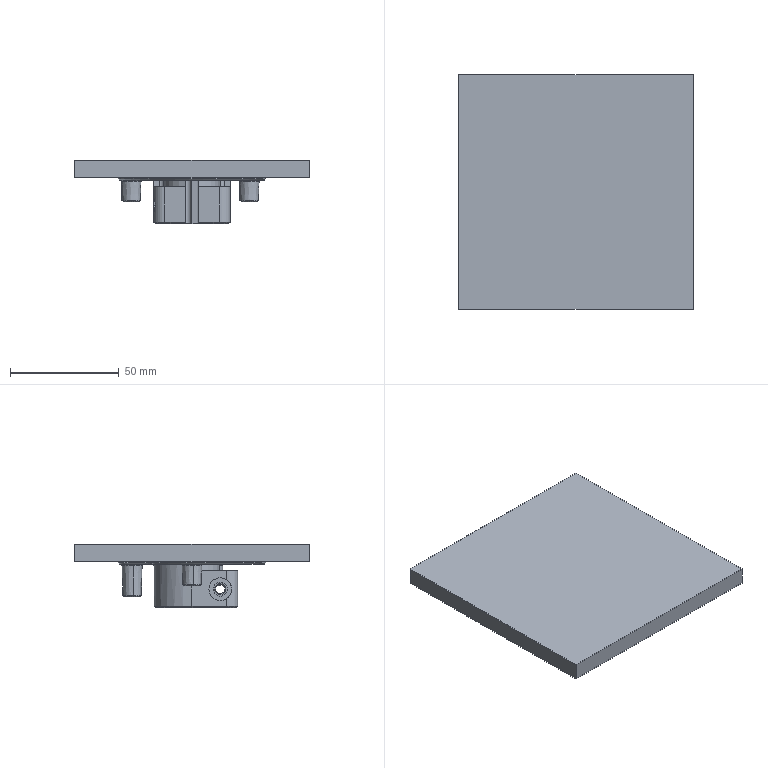NC program | NX | posted with a generic post | part box 108 x 108 x 29 mm
Lines 2749 to 3590 of 13118:
(ZLEVEL_PROFILE_COPY_COPY_COPY_1_COPY_COPY_1 , TOOL : D6JING)
N5466 T16 M6
N5468 G54
N5470 G17 G0 G90 X-1.747 Y-5.057 S9500 M3
N5472 G43 Z30. H16
N5474 Z-1.2
N5476 G94 G1 X-1.761 Y-5.965 F1000.
N5478 G3 X-1.468 Y-6.489 R0.6
N5480 G2 X0. Y-9.068 R3.013 F1500.
N5482 G1 X0.004 Y-9.036
N5484 X0.019 Y-8.767
N5486 X0.016 Y-8.756
N5488 G2 X1.421 Y-6.516 R3.
N5490 G3 X1.705 Y-5.987 R0.6
N5492 G1 X1.678 Y-5.08
N5494 G0 X-1.747 Y-5.057 Z-1.6
N5496 G1 X-1.761 Y-5.965 F1000.
N5498 G3 X-1.468 Y-6.489 R0.6
N5500 G2 X0. Y-9.068 R3.013 F1500.
N5502 G1 X0.004 Y-9.036
N5504 X0.019 Y-8.767
N5506 X0.016 Y-8.756
N5508 G2 X1.421 Y-6.515 R3.
N5510 G3 X1.706 Y-5.987 R0.6
N5512 G1 X1.678 Y-5.08
N5514 G0 X-1.747 Y-5.057 Z-2.
N5516 G1 X-1.76 Y-5.965 F1000.
N5518 G3 X-1.468 Y-6.489 R0.6
N5520 G2 X0. Y-9.068 R3.013 F1500.
N5522 G1 X0.004 Y-9.036
N5524 X0.019 Y-8.767
N5526 X0.016 Y-8.756
N5528 G2 X1.422 Y-6.515 R3.
N5530 G3 X1.706 Y-5.987 R0.6
N5532 G1 X1.678 Y-5.08
N5534 G0 X-1.747 Y-5.057 Z-2.4
N5536 G1 X-1.76 Y-5.965 F1000.
N5538 G3 X-1.468 Y-6.489 R0.6
N5540 G2 X0. Y-9.068 R3.013 F1500.
N5542 G1 X0.004 Y-9.036
N5544 X0.019 Y-8.767
N5546 X0.016 Y-8.756
N5548 G2 X1.422 Y-6.515 R3.
N5550 G3 X1.706 Y-5.987 R0.6
N5552 G1 X1.678 Y-5.08
N5554 G0 X-1.747 Y-5.057 Z-2.8
N5556 G1 X-1.76 Y-5.965 F1000.
N5558 G3 X-1.468 Y-6.489 R0.6
N5560 G2 X0. Y-9.068 R3.012 F1500.
N5562 G1 X0.004 Y-9.036
N5564 X0.018 Y-8.767
N5566 X0.016 Y-8.756
N5568 G2 X1.422 Y-6.515 R3.
N5570 G3 X1.706 Y-5.987 R0.6
N5572 G1 X1.679 Y-5.08
N5574 G0 X-1.747 Y-5.057 Z-3.2
N5576 G1 X-1.76 Y-5.965 F1000.
N5578 G3 X-1.468 Y-6.489 R0.6
N5580 G2 X0. Y-9.068 R3.012 F1500.
N5582 G1 X0.004 Y-9.036
N5584 X0.018 Y-8.767
N5586 X0.016 Y-8.756
N5588 G2 X1.422 Y-6.515 R3.
N5590 G3 X1.706 Y-5.987 R0.6
N5592 G1 X1.679 Y-5.08
N5594 G0 X-1.73 Y-5.062 Z-3.6
N5596 G1 X-1.746 Y-5.97 F1000.
N5598 G3 X-1.455 Y-6.495 R0.6
N5600 G2 X-0.016 Y-8.853 R2.983 F1500.
N5602 G1 X-0.001 Y-9.056
N5604 X0.003 Y-8.93
N5606 G2 X1.422 Y-6.515 R3.
N5608 G3 X1.706 Y-5.987 R0.6
N5610 G1 X1.679 Y-5.08
N5612 G0 X-1.73 Y-5.062 Z-4.
N5614 G1 X-1.746 Y-5.97 F1000.
N5616 G3 X-1.455 Y-6.495 R0.6
N5618 G2 X-0.016 Y-8.853 R2.983 F1500.
N5620 G1 X-0.001 Y-9.056
N5622 X0.003 Y-8.929
N5624 G2 X1.422 Y-6.515 R3.
N5626 G3 X1.707 Y-5.986 R0.6
N5628 G1 X1.679 Y-5.08
N5630 G0 X-1.73 Y-5.062 Z-4.4
N5632 G1 X-1.746 Y-5.97 F1000.
N5634 G3 X-1.455 Y-6.495 R0.6
N5636 G2 X-0.016 Y-8.853 R2.983 F1500.
N5638 G1 X-0.001 Y-9.056
N5640 X0.003 Y-8.928
N5642 G2 X1.422 Y-6.515 R3.
N5644 G3 X1.707 Y-5.986 R0.6
N5646 G1 X1.679 Y-5.08
N5648 G0 X-1.73 Y-5.062 Z-4.8
N5650 G1 X-1.746 Y-5.97 F1000.
N5652 G3 X-1.455 Y-6.495 R0.6
N5654 G2 X-0.016 Y-8.853 R2.983 F1500.
N5656 G1 X-0.001 Y-9.056
N5658 X0.003 Y-8.927
N5660 G2 X1.423 Y-6.515 R3.
N5662 G3 X1.707 Y-5.986 R0.6
N5664 G1 X1.68 Y-5.079
N5666 G0 X-1.73 Y-5.062 Z-5.2
N5668 G1 X-1.746 Y-5.97 F1000.
N5670 G3 X-1.455 Y-6.494 R0.6
N5672 G2 X-0.015 Y-8.853 R2.983 F1500.
N5674 G1 X-0.001 Y-9.056
N5676 X0.003 Y-8.925
N5678 G2 X1.423 Y-6.515 R3.
N5680 G3 X1.707 Y-5.986 R0.6
N5682 G1 X1.68 Y-5.079
N5684 G0 X-1.73 Y-5.062 Z-5.6
N5686 G1 X-1.746 Y-5.97 F1000.
N5688 G3 X-1.455 Y-6.494 R0.6
N5690 G2 X-0.015 Y-8.853 R2.983 F1500.
N5692 G1 X-0.001 Y-9.054
N5694 X0.004 Y-8.914
N5696 G2 X1.423 Y-6.515 R3.
N5698 G3 X1.707 Y-5.986 R0.6
N5700 G1 X1.68 Y-5.079
N5702 G0 X-1.73 Y-5.062 Z-6.
N5704 G1 X-1.746 Y-5.97 F1000.
N5706 G3 X-1.455 Y-6.494 R0.6
N5708 G2 X-0.015 Y-8.853 R2.983 F1500.
N5710 G1 X-0.001 Y-9.054
N5712 X0.004 Y-8.913
N5714 G2 X1.423 Y-6.514 R3.
N5716 G3 X1.707 Y-5.986 R0.6
N5718 G1 X1.68 Y-5.079
N5720 G0 X-1.731 Y-5.062 Z-6.4
N5722 G1 X-1.746 Y-5.97 F1000.
N5724 G3 X-1.455 Y-6.494 R0.6
N5726 G2 X-0.015 Y-8.853 R2.983 F1500.
N5728 G1 X-0.001 Y-9.054
N5730 X0.004 Y-8.912
N5732 G2 X1.423 Y-6.514 R3.
N5734 G3 X1.708 Y-5.986 R0.6
N5736 G1 X1.681 Y-5.079
N5738 G0 X-1.731 Y-5.062 Z-6.8
N5740 G1 X-1.746 Y-5.97 F1000.
N5742 G3 X-1.455 Y-6.494 R0.6
N5744 G2 X-0.015 Y-8.853 R2.983 F1500.
N5746 G1 X-0.001 Y-9.054
N5748 X0.004 Y-8.91
N5750 G2 X1.423 Y-6.514 R3.
N5752 G3 X1.708 Y-5.986 R0.6
N5754 G1 X1.681 Y-5.079
N5756 G0 X-1.731 Y-5.062 Z-7.2
N5758 G1 X-1.746 Y-5.97 F1000.
N5760 G3 X-1.455 Y-6.494 R0.6
N5762 G2 X-0.015 Y-8.853 R2.983 F1500.
N5764 G1 X-0.001 Y-9.053
N5766 X0.004 Y-8.908
N5768 G2 X1.424 Y-6.514 R3.
N5770 G3 X1.708 Y-5.986 R0.6
N5772 G1 X1.681 Y-5.079
N5774 G0 X-1.728 Y-5.063 Z-7.6
N5776 G1 X-1.744 Y-5.971 F1000.
N5778 G3 X-1.453 Y-6.495 R0.6
N5780 G2 X-0.013 Y-8.832 R2.988 F1500.
N5782 X-0.001 Y-9.06 R5.117
N5784 G1 X0.004 Y-8.915
N5786 G2 X1.424 Y-6.514 R3.
N5788 G3 X1.708 Y-5.986 R0.6
N5790 G1 X1.681 Y-5.079
N5792 G0 X-1.728 Y-5.063 Z-8.
N5794 G1 X-1.744 Y-5.971 F1000.
N5796 G3 X-1.453 Y-6.495 R0.6
N5798 G2 X-0.013 Y-8.833 R2.988 F1500.
N5800 X-0.001 Y-9.059 R5.079
N5802 G1 X0.004 Y-8.912
N5804 G2 X1.424 Y-6.514 R3.
N5806 G3 X1.708 Y-5.986 R0.6
N5808 G1 X1.681 Y-5.079
N5810 G0 X-1.728 Y-5.063 Z-8.4
N5812 G1 X-1.744 Y-5.971 F1000.
N5814 G3 X-1.454 Y-6.495 R0.6
N5816 G2 X-0.013 Y-8.833 R2.989 F1500.
N5818 X-0.001 Y-9.059 R5.041
N5820 G1 X0.004 Y-8.909
N5822 G2 X1.424 Y-6.514 R3.
N5824 G3 X1.708 Y-5.986 R0.6
N5826 G1 X1.682 Y-5.079
N5828 G0 X-1.728 Y-5.063 Z-8.8
N5830 G1 X-1.744 Y-5.97 F1000.
N5832 G3 X-1.454 Y-6.495 R0.6
N5834 G2 X-0.013 Y-8.833 R2.989 F1500.
N5836 X-0.001 Y-9.058 R5.003
N5838 G1 X0.004 Y-8.907
N5840 G2 X1.424 Y-6.514 R3.
N5842 G3 X1.709 Y-5.986 R0.6
N5844 G1 X1.682 Y-5.079
N5846 G0 X-1.729 Y-5.063 Z-9.2
N5848 G1 X-1.745 Y-5.97 F1000.
N5850 G3 X-1.454 Y-6.495 R0.6
N5852 G2 X-0.013 Y-8.834 R2.989 F1500.
N5854 X-0.001 Y-9.058 R4.964
N5856 G1 X0.004 Y-8.904
N5858 G2 X1.424 Y-6.514 R3.
N5860 G3 X1.709 Y-5.986 R0.6
N5862 G1 X1.682 Y-5.079
N5864 G0 X-1.729 Y-5.063 Z-9.6
N5866 G1 X-1.745 Y-5.97 F1000.
N5868 G3 X-1.454 Y-6.495 R0.6
N5870 G2 X-0.013 Y-8.834 R2.989 F1500.
N5872 X-0.001 Y-9.057 R4.926
N5874 G1 X0.005 Y-8.901
N5876 G2 X1.424 Y-6.514 R3.
N5878 G3 X1.709 Y-5.985 R0.6
N5880 G1 X1.682 Y-5.079
N5882 G0 X-1.729 Y-5.063 Z-10.
N5884 G1 X-1.745 Y-5.97 F1000.
N5886 G3 X-1.454 Y-6.495 R0.6
N5888 G2 X-0.013 Y-8.834 R2.989 F1500.
N5890 X-0.001 Y-9.057 R4.887
N5892 G1 X0.005 Y-8.899
N5894 G2 X1.425 Y-6.514 R3.
N5896 G3 X1.709 Y-5.985 R0.6
N5898 G1 X1.683 Y-5.079
N5900 G0 X-1.736 Y-5.061 Z-10.4
N5902 G1 X-1.751 Y-5.968 F1000.
N5904 G3 X-1.459 Y-6.493 R0.6
N5906 G2 X-0.012 Y-8.843 R2.994 F1500.
N5908 X-0.001 Y-9.057 R4.848
N5910 G1 X0.005 Y-8.896
N5912 G2 X1.425 Y-6.513 R3.
N5914 G3 X1.709 Y-5.985 R0.6
N5916 G1 X1.683 Y-5.078
N5918 G0 X-1.736 Y-5.061 Z-10.8
N5920 G1 X-1.751 Y-5.968 F1000.
N5922 G3 X-1.459 Y-6.493 R0.6
N5924 G2 X-0.012 Y-8.843 R2.994 F1500.
N5926 X-0.001 Y-9.056 R4.808
N5928 G1 X0.005 Y-8.893
N5930 G2 X1.425 Y-6.513 R3.
N5932 G3 X1.71 Y-5.985 R0.6
N5934 G1 X1.683 Y-5.078
N5936 G0 X-1.736 Y-5.061 Z-11.2
N5938 G1 X-1.751 Y-5.968 F1000.
N5940 G3 X-1.459 Y-6.493 R0.6
N5942 G2 X-0.012 Y-8.844 R2.994 F1500.
N5944 X-0.001 Y-9.056 R4.769
N5946 G1 X0.005 Y-8.891
N5948 G2 X1.425 Y-6.513 R3.
N5950 G3 X1.71 Y-5.985 R0.6
N5952 G1 X1.683 Y-5.078
N5954 G0 X-1.736 Y-5.06 Z-11.6
N5956 G1 X-1.751 Y-5.968 F1000.
N5958 G3 X-1.459 Y-6.493 R0.6
N5960 G2 X-0.012 Y-8.844 R2.994 F1500.
N5962 X-0.001 Y-9.056 R4.729
N5964 G1 X0.005 Y-8.89
N5966 G2 X1.425 Y-6.513 R3.
N5968 G3 X1.71 Y-5.985 R0.6
N5970 G1 X1.683 Y-5.078
N5972 G0 X-1.736 Y-5.06 Z-12.
N5974 G1 X-1.751 Y-5.968 F1000.
N5976 G3 X-1.459 Y-6.493 R0.6
N5978 G2 X-0.012 Y-8.845 R2.994 F1500.
N5980 X-0.001 Y-9.054 R4.69
N5982 G1 X0.006 Y-8.879
N5984 G2 X1.425 Y-6.513 R3.
N5986 G3 X1.71 Y-5.985 R0.6
N5988 G1 X1.684 Y-5.078
N5990 G0 X-1.736 Y-5.06 Z-12.4
N5992 G1 X-1.751 Y-5.968 F1000.
N5994 G3 X-1.459 Y-6.492 R0.6
N5996 G2 X-0.012 Y-8.845 R2.994 F1500.
N5998 X-0.001 Y-9.055 R4.649
N6000 G1 X0.006 Y-8.879
N6002 G2 X1.425 Y-6.513 R3.
N6004 G3 X1.71 Y-5.985 R0.6
N6006 G1 X1.684 Y-5.078
N6008 G0 X-1.736 Y-5.06 Z-12.8
N6010 G1 X-1.751 Y-5.968 F1000.
N6012 G3 X-1.459 Y-6.492 R0.6
N6014 G2 X-0.012 Y-8.845 R2.994 F1500.
N6016 X-0.001 Y-9.055 R4.609
N6018 G1 X0.006 Y-8.879
N6020 G2 X1.426 Y-6.513 R3.
N6022 G3 X1.71 Y-5.985 R0.6
N6024 G1 X1.684 Y-5.078
N6026 G0 X-1.778 Y-5.046 Z-13.2
N6028 G1 X-1.786 Y-5.956 F1000.
N6030 G3 X-1.491 Y-6.478 R0.6
N6032 G2 X0.001 Y-8.973 R3.033 F1500.
N6034 G1 X0.006 Y-8.881
N6036 G2 X1.426 Y-6.513 R3.
N6038 G3 X1.711 Y-5.985 R0.6
N6040 G1 X1.684 Y-5.078
N6042 G0 X-1.766 Y-5.05 Z-13.6
N6044 G1 X-1.776 Y-5.96 F1000.
N6046 G3 X-1.481 Y-6.482 R0.6
N6048 G2 X0.001 Y-8.971 R3.025 F1500.
N6050 G1 X0.006 Y-8.881
N6052 G2 X1.426 Y-6.513 R3.
N6054 G3 X1.711 Y-5.985 R0.6
N6056 G1 X1.685 Y-5.078
N6058 G0 X-1.745 Y-5.057 Z-14.
N6060 G1 X-1.758 Y-5.966 F1000.
N6062 G3 X-1.466 Y-6.49 R0.6
N6064 G2 X0. Y-9.067 R3.006 F1500.
N6066 G1 X0.017 Y-8.767
N6068 X0.016 Y-8.756
N6070 G2 X1.426 Y-6.513 R3.
N6072 G3 X1.711 Y-5.985 R0.6
N6074 G1 X1.685 Y-5.078
N6076 G0 X-1.745 Y-5.057 Z-14.4
N6078 G1 X-1.758 Y-5.966 F1000.
N6080 G3 X-1.465 Y-6.49 R0.6
N6082 G2 X0. Y-9.067 R3.006 F1500.
N6084 G1 X0.017 Y-8.767
N6086 X0.016 Y-8.756
N6088 G2 X1.426 Y-6.513 R3.
N6090 G3 X1.711 Y-5.985 R0.6
N6092 G1 X1.685 Y-5.078
N6094 G0 X-1.745 Y-5.058 Z-14.8
N6096 G1 X-1.758 Y-5.966 F1000.
N6098 G3 X-1.465 Y-6.49 R0.6
N6100 G2 X0. Y-9.067 R3.006 F1500.
N6102 G1 X0.017 Y-8.767
N6104 X0.016 Y-8.756
N6106 G2 X1.426 Y-6.512 R3.
N6108 G3 X1.711 Y-5.984 R0.6
N6110 G1 X1.685 Y-5.078
N6112 G0 X-1.745 Y-5.058 Z-15.2
N6114 G1 X-1.758 Y-5.966 F1000.
N6116 G3 X-1.465 Y-6.49 R0.6
N6118 G2 X0. Y-9.067 R3.006 F1500.
N6120 G1 X0.016 Y-8.756
N6122 G2 X1.426 Y-6.512 R3.
N6124 G3 X1.711 Y-5.984 R0.6
N6126 G1 X1.686 Y-5.078
N6128 G0 X-1.745 Y-5.058 Z-15.6
N6130 G1 X-1.758 Y-5.966 F1000.
N6132 G3 X-1.465 Y-6.49 R0.6
N6134 G2 X0. Y-9.067 R3.005 F1500.
N6136 G1 X0.016 Y-8.756
N6138 G2 X1.427 Y-6.512 R3.
N6140 G3 X1.712 Y-5.984 R0.6
N6142 G1 X1.686 Y-5.077
N6144 G0 X-1.745 Y-5.058 Z-16.
N6146 G1 X-1.758 Y-5.966 F1000.
N6148 G3 X-1.465 Y-6.49 R0.6
N6150 G2 X0. Y-9.066 R3.005 F1500.
N6152 G1 X0.016 Y-8.756
N6154 G2 X1.427 Y-6.512 R3.
N6156 G3 X1.712 Y-5.984 R0.6
N6158 G1 X1.686 Y-5.077
N6160 G0 X-1.744 Y-5.058 Z-16.4
N6162 G1 X-1.758 Y-5.966 F1000.
N6164 G3 X-1.465 Y-6.49 R0.6
N6166 G2 X0. Y-9.066 R3.005 F1500.
N6168 G1 X0.016 Y-8.756
N6170 G2 X1.427 Y-6.512 R3.
N6172 G3 X1.712 Y-5.984 R0.6
N6174 G1 X1.686 Y-5.077
N6176 G0 X-1.744 Y-5.058 Z-16.8
N6178 G1 X-1.757 Y-5.966 F1000.
N6180 G3 X-1.465 Y-6.49 R0.6
N6182 G2 X0. Y-9.066 R3.005 F1500.
N6184 G1 X0.016 Y-8.756
N6186 G2 X1.427 Y-6.512 R3.
N6188 G3 X1.712 Y-5.984 R0.6
N6190 G1 X1.686 Y-5.077
N6192 G0 X-1.744 Y-5.058 Z-17.2
N6194 G1 X-1.757 Y-5.966 F1000.
N6196 G3 X-1.465 Y-6.49 R0.6
N6198 G2 X0. Y-9.066 R3.004 F1500.
N6200 G1 X0.016 Y-8.756
N6202 G2 X1.427 Y-6.512 R3.
N6204 G3 X1.712 Y-5.984 R0.6
N6206 G1 X1.687 Y-5.077
N6208 G0 X-1.744 Y-5.058 Z-17.6
N6210 G1 X-1.757 Y-5.966 F1000.
N6212 G3 X-1.465 Y-6.49 R0.6
N6214 G2 X0. Y-9.066 R3.004 F1500.
N6216 G1 X0.016 Y-8.756
N6218 G2 X1.427 Y-6.512 R3.
N6220 G3 X1.713 Y-5.984 R0.6
N6222 G1 X1.687 Y-5.077
N6224 G0 X-1.744 Y-5.058 Z-18.
N6226 G1 X-1.757 Y-5.966 F1000.
N6228 G3 X-1.465 Y-6.49 R0.6
N6230 G2 X0. Y-9.066 R3.004 F1500.
N6232 G1 X0.016 Y-8.756
N6234 G2 X1.427 Y-6.512 R3.
N6236 G3 X1.713 Y-5.984 R0.6
N6238 G1 X1.687 Y-5.077
N6240 G0 X-1.744 Y-5.058 Z-18.4
N6242 G1 X-1.757 Y-5.966 F1000.
N6244 G3 X-1.465 Y-6.49 R0.6
N6246 G2 X0. Y-9.066 R3.004 F1500.
N6248 G1 X0.016 Y-8.756
N6250 G2 X1.428 Y-6.512 R3.
N6252 G3 X1.713 Y-5.984 R0.6
N6254 G1 X1.687 Y-5.077
N6256 G0 X-1.744 Y-5.058 Z-18.8
N6258 G1 X-1.757 Y-5.966 F1000.
N6260 G3 X-1.465 Y-6.49 R0.6
N6262 G2 X0. Y-9.066 R3.004 F1500.
N6264 G1 X0.016 Y-8.756
N6266 G2 X1.428 Y-6.512 R3.
N6268 G3 X1.713 Y-5.984 R0.6
N6270 G1 X1.688 Y-5.077
N6272 G0 X-1.744 Y-5.058 Z-19.2
N6274 G1 X-1.757 Y-5.966 F1000.
N6276 G3 X-1.464 Y-6.49 R0.6
N6278 G2 X0. Y-9.066 R3.003 F1500.
N6280 G1 X0.016 Y-8.756
N6282 G2 X1.428 Y-6.511 R3.
N6284 G3 X1.713 Y-5.984 R0.6
N6286 G1 X1.688 Y-5.077
N6288 G0 X-1.744 Y-5.058 Z-19.6
N6290 G1 X-1.757 Y-5.966 F1000.
N6292 G3 X-1.464 Y-6.49 R0.6
N6294 G2 X0. Y-9.066 R3.003 F1500.
N6296 G1 X0.016 Y-8.756
N6298 G2 X1.428 Y-6.511 R3.
N6300 G3 X1.713 Y-5.984 R0.6
N6302 G1 X1.688 Y-5.077
N6304 G0 X-1.744 Y-5.058 Z-20.
N6306 G1 X-1.757 Y-5.966 F1000.
N6308 G3 X-1.464 Y-6.49 R0.6
N6310 G2 X0. Y-9.066 R3.003 F1500.
N6312 G1 X0.016 Y-8.756
N6314 G2 X1.428 Y-6.511 R3.
N6316 G3 X1.714 Y-5.984 R0.6
N6318 G1 X1.688 Y-5.077
N6320 G0 X-1.744 Y-5.058 Z-20.4
N6322 G1 X-1.757 Y-5.966 F1000.
N6324 G3 X-1.464 Y-6.49 R0.6
N6326 G2 X0. Y-9.066 R3.003 F1500.
N6328 G1 X0.001 Y-9.036
N6330 X0.016 Y-8.756
N6332 G2 X1.428 Y-6.511 R3.
N6334 G3 X1.714 Y-5.983 R0.6
N6336 G1 X1.689 Y-5.077
N6338 G0 X-1.744 Y-5.058 Z-20.8
N6340 G1 X-1.757 Y-5.966 F1000.
N6342 G3 X-1.464 Y-6.49 R0.6
N6344 G2 X0. Y-9.066 R3.002 F1500.
N6346 G1 X0.001 Y-9.036
N6348 X0.016 Y-8.756
N6350 G2 X1.428 Y-6.511 R3.
N6352 G3 X1.714 Y-5.983 R0.6
N6354 G1 X1.689 Y-5.076
N6356 G0 X-1.744 Y-5.058 Z-21.2
N6358 G1 X-1.757 Y-5.966 F1000.
N6360 G3 X-1.464 Y-6.49 R0.6
N6362 G2 X0. Y-9.066 R3.002 F1500.
N6364 G1 X0.001 Y-9.036
N6366 X0.016 Y-8.756
N6368 G2 X1.429 Y-6.511 R3.
N6370 G3 X1.714 Y-5.983 R0.6
N6372 G1 X1.689 Y-5.076
N6374 G0 X-1.744 Y-5.058 Z-21.6
N6376 G1 X-1.757 Y-5.966 F1000.
N6378 G3 X-1.464 Y-6.49 R0.6
N6380 G2 X0. Y-9.066 R3.002 F1500.
N6382 G1 X0.001 Y-9.036
N6384 X0.016 Y-8.756
N6386 G2 X1.429 Y-6.511 R3.
N6388 G3 X1.714 Y-5.983 R0.6
N6390 G1 X1.689 Y-5.076
N6392 G0 X-1.744 Y-5.058 Z-22.
N6394 G1 X-1.757 Y-5.966 F1000.
N6396 G3 X-1.464 Y-6.49 R0.6
N6398 G2 X0. Y-9.066 R3.002 F1500.
N6400 G1 X0.001 Y-9.036
N6402 X0.016 Y-8.756
N6404 G2 X1.429 Y-6.511 R3.
N6406 G3 X1.714 Y-5.983 R0.6
N6408 G1 X1.689 Y-5.076
N6410 G0 X-1.744 Y-5.058 Z-22.4
N6412 G1 X-1.757 Y-5.966 F1000.
N6414 G3 X-1.464 Y-6.49 R0.6
N6416 G2 X0. Y-9.066 R3.002 F1500.
N6418 G1 X0.001 Y-9.036
N6420 X0.016 Y-8.756
N6422 G2 X1.429 Y-6.511 R3.
N6424 G3 X1.715 Y-5.983 R0.6
N6426 G1 X1.69 Y-5.076
N6428 G0 X-1.744 Y-5.058 Z-22.8
N6430 G1 X-1.757 Y-5.966 F1000.
N6432 G3 X-1.464 Y-6.49 R0.6
N6434 G2 X0. Y-9.066 R3.002 F1500.
N6436 G1 X0.001 Y-9.036
N6438 X0.016 Y-8.756
N6440 G2 X1.429 Y-6.511 R3.
N6442 G3 X1.715 Y-5.983 R0.6
N6444 G1 X1.69 Y-5.076
N6446 G0 X-1.744 Y-5.058 Z-23.2
N6448 G1 X-1.757 Y-5.966 F1000.
N6450 G3 X-1.464 Y-6.49 R0.6
N6452 G2 X0. Y-9.066 R3.001 F1500.
N6454 G1 X0.001 Y-9.036
N6456 X0.016 Y-8.756
N6458 G2 X1.429 Y-6.511 R3.
N6460 G3 X1.715 Y-5.983 R0.6
N6462 G1 X1.69 Y-5.076
N6464 G0 X-1.743 Y-5.058 Z-23.6
N6466 G1 X-1.756 Y-5.966 F1000.
N6468 G3 X-1.463 Y-6.49 R0.6
N6470 G2 X0. Y-9.066 R3.001 F1500.
N6472 G1 Y-9.036
N6474 X0.016 Y-8.756
N6476 G2 X1.43 Y-6.51 R3.
N6478 G3 X1.715 Y-5.983 R0.6
N6480 G1 X1.69 Y-5.076
N6482 G0 X-1.743 Y-5.058 Z-23.95
N6484 G1 X-1.756 Y-5.966 F1000.
N6486 G3 X-1.463 Y-6.49 R0.6
N6488 G2 X0. Y-9.066 R3. F1500.
N6490 G1 Y-9.036
N6492 X0.016 Y-8.756
N6494 G2 X1.43 Y-6.51 R3.
N6496 G3 X1.715 Y-5.983 R0.6
N6498 G1 X1.691 Y-5.076
N6500 G0 X-1.743 Y-5.058 Z-24.3
N6502 G1 X-1.756 Y-5.966 F1000.
N6504 G3 X-1.463 Y-6.49 R0.6
N6506 G2 X0. Y-9.066 R3. F1500.
N6508 G1 Y-9.036
N6510 X0.016 Y-8.756
N6512 G2 X1.43 Y-6.51 R3.
N6514 G3 X1.715 Y-5.983 R0.6
N6516 G1 X1.691 Y-5.076
N6518 G0 X-1.743 Y-5.058 Z-24.65
N6520 G1 X-1.756 Y-5.966 F1000.
N6522 G3 X-1.463 Y-6.49 R0.6
N6524 G2 X0. Y-9.036 R3.001 F1500.
N6526 G1 X0.016 Y-8.756
N6528 G2 X1.43 Y-6.51 R3.
N6530 G3 X1.716 Y-5.983 R0.6
N6532 G1 X1.691 Y-5.076
N6534 G0 X-1.743 Y-5.058 Z-25.
N6536 G1 X-1.756 Y-5.966 F1000.
N6538 G3 X-1.463 Y-6.49 R0.6
N6540 G2 X0. Y-9.036 R3. F1500.
N6542 G1 X0.016 Y-8.756
N6544 G2 X1.43 Y-6.51 R3.
N6546 G3 X1.716 Y-5.983 R0.6
N6548 G1 X1.691 Y-5.076
N6550 G0 Z30.
N6552 X0.735 Y5.299
N6554 Z-1.2
N6556 G1 X0.264 Y6.227 F1000.
N6558 G3 X-0.239 Y6.554 R0.6
N6560 G2 X-1.193 Y6.764 R3. F1500.
N6562 X-2.017 Y6.24 R3.
N6564 G3 X-2.378 Y5.761 R0.6
N6566 G1 X-2.504 Y4.728
N6568 G0 X0.735 Y5.299 Z-1.6
N6570 G1 X0.264 Y6.227 F1000.
N6572 G3 X-0.239 Y6.554 R0.6
N6574 G2 X-1.193 Y6.764 R3. F1500.
N6576 X-2.017 Y6.24 R3.
N6578 G3 X-2.378 Y5.761 R0.6
N6580 G1 X-2.504 Y4.728
N6582 G0 X0.735 Y5.299 Z-2.
N6584 G1 X0.264 Y6.227 F1000.
N6586 G3 X-0.239 Y6.554 R0.6
N6588 G2 X-1.193 Y6.764 R3. F1500.
N6590 X-2.017 Y6.24 R3.
N6592 G3 X-2.378 Y5.761 R0.6
N6594 G1 X-2.504 Y4.728
N6596 G0 X0.735 Y5.299 Z-2.4
N6598 G1 X0.264 Y6.227 F1000.
N6600 G3 X-0.239 Y6.554 R0.6
N6602 G2 X-1.193 Y6.764 R3. F1500.
N6604 X-2.017 Y6.24 R3.
N6606 G3 X-2.378 Y5.761 R0.6
N6608 G1 X-2.504 Y4.728
N6610 G0 X0.735 Y5.299 Z-2.8
N6612 G1 X0.264 Y6.227 F1000.
N6614 G3 X-0.239 Y6.554 R0.6
N6616 G2 X-1.193 Y6.764 R3. F1500.
N6618 X-2.017 Y6.24 R3.
N6620 G3 X-2.378 Y5.761 R0.6
N6622 G1 X-2.504 Y4.728
N6624 G0 X0.735 Y5.299 Z-3.2
N6626 G1 X0.264 Y6.227 F1000.
N6628 G3 X-0.239 Y6.554 R0.6
N6630 G2 X-1.193 Y6.764 R3. F1500.
N6632 X-2.017 Y6.24 R3.
N6634 G3 X-2.378 Y5.761 R0.6
N6636 G1 X-2.504 Y4.728
N6638 G0 X0.735 Y5.299 Z-3.6
N6640 G1 X0.264 Y6.227 F1000.
N6642 G3 X-0.239 Y6.554 R0.6
N6644 G2 X-1.193 Y6.764 R3. F1500.
N6646 X-2.017 Y6.24 R3.
N6648 G3 X-2.378 Y5.761 R0.6
N6650 G1 X-2.504 Y4.728
N6652 G0 X0.735 Y5.299 Z-4.
N6654 G1 X0.264 Y6.227 F1000.
N6656 G3 X-0.239 Y6.554 R0.6
N6658 G2 X-1.193 Y6.764 R3. F1500.
N6660 X-2.017 Y6.24 R3.
N6662 G3 X-2.378 Y5.761 R0.6
N6664 G1 X-2.504 Y4.728
N6666 G0 X0.735 Y5.299 Z-4.4
N6668 G1 X0.264 Y6.227 F1000.
N6670 G3 X-0.239 Y6.554 R0.6
N6672 G2 X-1.193 Y6.764 R3. F1500.
N6674 X-2.017 Y6.24 R3.
N6676 G3 X-2.378 Y5.761 R0.6
N6678 G1 X-2.504 Y4.728
N6680 G0 X0.735 Y5.299 Z-4.8
N6682 G1 X0.264 Y6.227 F1000.
N6684 G3 X-0.239 Y6.554 R0.6
N6686 G2 X-1.193 Y6.764 R3. F1500.
N6688 X-2.017 Y6.24 R3.
N6690 G3 X-2.378 Y5.761 R0.6
N6692 G1 X-2.504 Y4.728
N6694 G0 X0.735 Y5.299 Z-5.2
N6696 G1 X0.264 Y6.227 F1000.
N6698 G3 X-0.239 Y6.554 R0.6
N6700 G2 X-1.193 Y6.764 R3. F1500.
N6702 X-2.017 Y6.24 R3.
N6704 G3 X-2.378 Y5.761 R0.6
N6706 G1 X-2.504 Y4.728
N6708 G0 X0.735 Y5.299 Z-5.6
N6710 G1 X0.264 Y6.227 F1000.
N6712 G3 X-0.239 Y6.554 R0.6
N6714 G2 X-1.193 Y6.764 R3. F1500.
N6716 X-2.017 Y6.24 R3.
N6718 G3 X-2.378 Y5.761 R0.6
N6720 G1 X-2.504 Y4.728
N6722 G0 X0.735 Y5.299 Z-6.
N6724 G1 X0.264 Y6.227 F1000.
N6726 G3 X-0.239 Y6.554 R0.6
N6728 G2 X-1.193 Y6.764 R3. F1500.
N6730 X-2.017 Y6.24 R3.
N6732 G3 X-2.378 Y5.761 R0.6
N6734 G1 X-2.504 Y4.728
N6736 G0 X0.735 Y5.299 Z-6.4
N6738 G1 X0.264 Y6.227 F1000.
N6740 G3 X-0.239 Y6.554 R0.6
N6742 G2 X-1.193 Y6.764 R3. F1500.
N6744 X-2.017 Y6.24 R3.
N6746 G3 X-2.378 Y5.761 R0.6
N6748 G1 X-2.504 Y4.728
N6750 G0 X0.735 Y5.299 Z-6.8
N6752 G1 X0.264 Y6.227 F1000.
N6754 G3 X-0.239 Y6.554 R0.6
N6756 G2 X-1.193 Y6.764 R3. F1500.
N6758 X-2.017 Y6.24 R3.
N6760 G3 X-2.378 Y5.761 R0.6
N6762 G1 X-2.504 Y4.728
N6764 G0 X0.735 Y5.299 Z-7.2
N6766 G1 X0.264 Y6.227 F1000.
N6768 G3 X-0.239 Y6.554 R0.6
N6770 G2 X-1.193 Y6.764 R3. F1500.
N6772 X-2.017 Y6.24 R3.
N6774 G3 X-2.378 Y5.761 R0.6
N6776 G1 X-2.504 Y4.728
N6778 G0 X0.735 Y5.299 Z-7.6
N6780 G1 X0.264 Y6.227 F1000.
N6782 G3 X-0.239 Y6.554 R0.6
N6784 G2 X-1.193 Y6.764 R3. F1500.
N6786 X-2.017 Y6.24 R3.
N6788 G3 X-2.378 Y5.761 R0.6
N6790 G1 X-2.504 Y4.728
N6792 G0 X0.735 Y5.299 Z-8.
N6794 G1 X0.264 Y6.227 F1000.
N6796 G3 X-0.239 Y6.554 R0.6
N6798 G2 X-1.193 Y6.764 R3. F1500.
N6800 X-2.017 Y6.24 R3.
N6802 G3 X-2.378 Y5.761 R0.6
N6804 G1 X-2.504 Y4.728
N6806 G0 X0.735 Y5.299 Z-8.4
N6808 G1 X0.264 Y6.227 F1000.
N6810 G3 X-0.239 Y6.554 R0.6
N6812 G2 X-1.193 Y6.764 R3. F1500.
N6814 X-2.017 Y6.24 R3.
N6816 G3 X-2.378 Y5.761 R0.6
N6818 G1 X-2.504 Y4.728
N6820 G0 X0.735 Y5.299 Z-8.8
N6822 G1 X0.264 Y6.227 F1000.
N6824 G3 X-0.239 Y6.554 R0.6
N6826 G2 X-1.193 Y6.764 R3. F1500.
N6828 X-2.017 Y6.24 R3.
N6830 G3 X-2.378 Y5.761 R0.6
N6832 G1 X-2.504 Y4.728
N6834 G0 X0.735 Y5.299 Z-9.2
N6836 G1 X0.264 Y6.227 F1000.
N6838 G3 X-0.239 Y6.554 R0.6
N6840 G2 X-1.193 Y6.764 R3. F1500.
N6842 X-2.017 Y6.24 R3.
N6844 G3 X-2.378 Y5.761 R0.6
N6846 G1 X-2.504 Y4.728
N6848 G0 X0.735 Y5.299 Z-9.6
N6850 G1 X0.264 Y6.227 F1000.
N6852 G3 X-0.239 Y6.554 R0.6
N6854 G2 X-1.193 Y6.764 R3. F1500.
N6856 X-2.017 Y6.24 R3.
N6858 G3 X-2.378 Y5.761 R0.6
N6860 G1 X-2.504 Y4.728
N6862 G0 X0.735 Y5.299 Z-10.
N6864 G1 X0.264 Y6.227 F1000.
N6866 G3 X-0.239 Y6.554 R0.6
N6868 G2 X-1.193 Y6.764 R3. F1500.
N6870 X-2.017 Y6.24 R3.
N6872 G3 X-2.378 Y5.761 R0.6
N6874 G1 X-2.504 Y4.728
N6876 G0 X0.735 Y5.299 Z-10.4
N6878 G1 X0.264 Y6.227 F1000.
N6880 G3 X-0.239 Y6.554 R0.6
N6882 G2 X-1.193 Y6.764 R3. F1500.
N6884 X-2.017 Y6.24 R3.
N6886 G3 X-2.378 Y5.761 R0.6
N6888 G1 X-2.504 Y4.728
N6890 G0 X0.735 Y5.299 Z-10.8
N6892 G1 X0.264 Y6.227 F1000.
N6894 G3 X-0.239 Y6.554 R0.6
N6896 G2 X-1.193 Y6.764 R3. F1500.
N6898 X-2.017 Y6.24 R3.
N6900 G3 X-2.378 Y5.761 R0.6
N6902 G1 X-2.504 Y4.728
N6904 G0 X0.735 Y5.299 Z-11.2
N6906 G1 X0.264 Y6.227 F1000.
N6908 G3 X-0.239 Y6.554 R0.6
N6910 G2 X-1.193 Y6.764 R3. F1500.
N6912 X-2.017 Y6.24 R3.
N6914 G3 X-2.378 Y5.761 R0.6
N6916 G1 X-2.504 Y4.728
N6918 G0 X0.735 Y5.299 Z-11.6
N6920 G1 X0.264 Y6.227 F1000.
N6922 G3 X-0.239 Y6.554 R0.6
N6924 G2 X-1.193 Y6.764 R3. F1500.
N6926 X-2.017 Y6.24 R3.
N6928 G3 X-2.378 Y5.761 R0.6
N6930 G1 X-2.504 Y4.728
N6932 G0 X0.735 Y5.299 Z-12.
N6934 G1 X0.264 Y6.227 F1000.
N6936 G3 X-0.239 Y6.554 R0.6
N6938 G2 X-1.193 Y6.764 R3. F1500.
N6940 X-2.017 Y6.24 R3.
N6942 G3 X-2.378 Y5.761 R0.6
N6944 G1 X-2.504 Y4.728
N6946 G0 X0.735 Y5.299 Z-12.4
N6948 G1 X0.264 Y6.227 F1000.
N6950 G3 X-0.239 Y6.554 R0.6
N6952 G2 X-1.193 Y6.764 R3. F1500.
N6954 X-2.017 Y6.24 R3.
N6956 G3 X-2.378 Y5.761 R0.6
N6958 G1 X-2.504 Y4.728
N6960 G0 X0.735 Y5.299 Z-12.8
N6962 G1 X0.264 Y6.227 F1000.
N6964 G3 X-0.239 Y6.554 R0.6
N6966 G2 X-1.193 Y6.764 R3. F1500.
N6968 X-2.017 Y6.24 R3.
N6970 G3 X-2.378 Y5.761 R0.6
N6972 G1 X-2.504 Y4.728
N6974 G0 X0.735 Y5.299 Z-13.2
N6976 G1 X0.264 Y6.227 F1000.
N6978 G3 X-0.239 Y6.554 R0.6
N6980 G2 X-1.193 Y6.764 R3. F1500.
N6982 X-2.017 Y6.24 R3.
N6984 G3 X-2.378 Y5.761 R0.6
N6986 G1 X-2.504 Y4.728
N6988 G0 X0.735 Y5.299 Z-13.6
N6990 G1 X0.264 Y6.227 F1000.
N6992 G3 X-0.239 Y6.554 R0.6
N6994 G2 X-1.193 Y6.764 R3. F1500.
N6996 X-2.017 Y6.24 R3.
N6998 G3 X-2.378 Y5.761 R0.6
N7000 G1 X-2.504 Y4.728
N7002 G0 X0.735 Y5.299 Z-14.
N7004 G1 X0.264 Y6.227 F1000.
N7006 G3 X-0.239 Y6.554 R0.6
N7008 G2 X-1.193 Y6.764 R3. F1500.
N7010 X-2.017 Y6.24 R3.
N7012 G3 X-2.378 Y5.761 R0.6
N7014 G1 X-2.504 Y4.728
N7016 G0 X0.735 Y5.299 Z-14.4
N7018 G1 X0.264 Y6.227 F1000.
N7020 G3 X-0.239 Y6.554 R0.6
N7022 G2 X-1.193 Y6.764 R3. F1500.
N7024 X-2.017 Y6.24 R3.
N7026 G3 X-2.378 Y5.761 R0.6
N7028 G1 X-2.504 Y4.728
N7030 G0 X0.735 Y5.299 Z-14.8
N7032 G1 X0.264 Y6.227 F1000.
N7034 G3 X-0.239 Y6.554 R0.6
N7036 G2 X-1.193 Y6.764 R3. F1500.
N7038 X-2.017 Y6.24 R3.
N7040 G3 X-2.378 Y5.761 R0.6
N7042 G1 X-2.504 Y4.728
N7044 G0 X0.735 Y5.299 Z-15.2
N7046 G1 X0.264 Y6.227 F1000.
N7048 G3 X-0.239 Y6.554 R0.6
N7050 G2 X-1.193 Y6.764 R3. F1500.
N7052 X-2.017 Y6.24 R3.
N7054 G3 X-2.378 Y5.761 R0.6
N7056 G1 X-2.504 Y4.728
N7058 G0 X0.735 Y5.299 Z-15.6
N7060 G1 X0.264 Y6.227 F1000.
N7062 G3 X-0.239 Y6.554 R0.6
N7064 G2 X-1.193 Y6.764 R3. F1500.
N7066 X-2.017 Y6.24 R3.
N7068 G3 X-2.378 Y5.761 R0.6
N7070 G1 X-2.504 Y4.728
N7072 G0 X0.735 Y5.299 Z-16.
N7074 G1 X0.264 Y6.227 F1000.
N7076 G3 X-0.239 Y6.554 R0.6
N7078 G2 X-1.193 Y6.764 R3. F1500.
N7080 X-2.017 Y6.24 R3.
N7082 G3 X-2.378 Y5.761 R0.6
N7084 G1 X-2.504 Y4.728
N7086 G0 X0.735 Y5.299 Z-16.4
N7088 G1 X0.264 Y6.227 F1000.
N7090 G3 X-0.239 Y6.554 R0.6
N7092 G2 X-1.193 Y6.764 R3. F1500.
N7094 X-2.017 Y6.24 R3.
N7096 G3 X-2.378 Y5.761 R0.6
N7098 G1 X-2.504 Y4.728
N7100 G0 X0.735 Y5.299 Z-16.8
N7102 G1 X0.264 Y6.227 F1000.
N7104 G3 X-0.239 Y6.554 R0.6
N7106 G2 X-1.193 Y6.764 R3. F1500.
N7108 X-2.017 Y6.24 R3.
N7110 G3 X-2.378 Y5.761 R0.6
N7112 G1 X-2.504 Y4.728
N7114 G0 X0.735 Y5.299 Z-17.2
N7116 G1 X0.264 Y6.227 F1000.
N7118 G3 X-0.239 Y6.554 R0.6
N7120 G2 X-1.193 Y6.764 R3. F1500.
N7122 X-2.017 Y6.24 R3.
N7124 G3 X-2.378 Y5.761 R0.6
N7126 G1 X-2.504 Y4.728
N7128 G0 X0.735 Y5.299 Z-17.6
N7130 G1 X0.264 Y6.227 F1000.
N7132 G3 X-0.239 Y6.554 R0.6
N7134 G2 X-1.193 Y6.764 R3. F1500.
N7136 X-2.017 Y6.24 R3.
N7138 G3 X-2.378 Y5.761 R0.6
N7140 G1 X-2.504 Y4.728
N7142 G0 X0.735 Y5.299 Z-18.